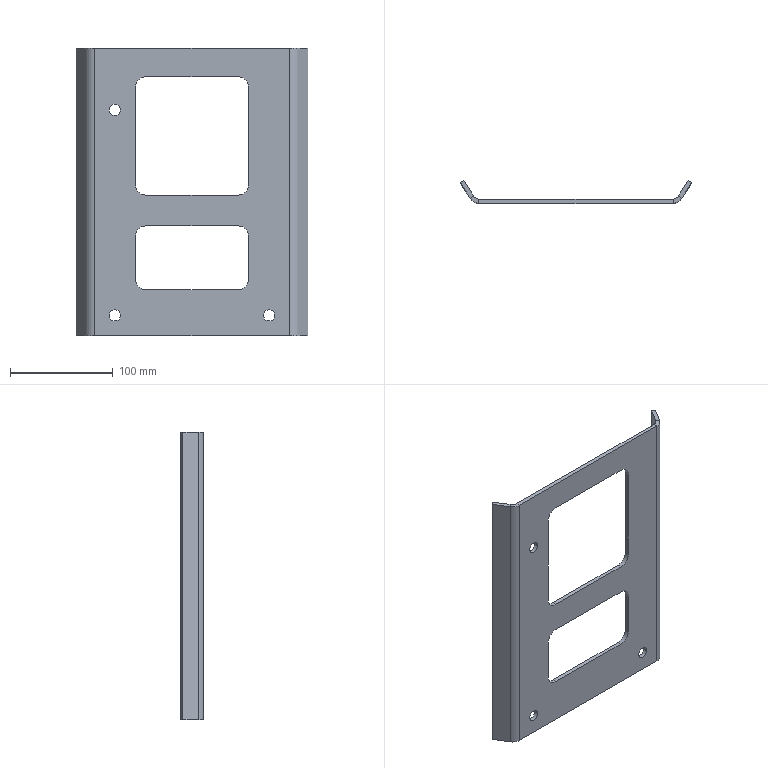Part | SolidWorks | features FlatPattern 1, ICE 1, SMBaseFlange 1, SheetMetal 1 | 1 solid | 44 faces | box 225 x 22.12 x 280 mm | volume 191805 mm3 | plane 26 | cylinder 18 | commonest cylinder face diameters 20 x10 11 x6 12 x2
STEP:
#1=CARTESIAN_POINT('',(182.,-16.,-120.));
#2=VERTEX_POINT('',#1);
#3=CARTESIAN_POINT('',(193.,-16.,-120.));
#4=VERTEX_POINT('',#3);
#5=CARTESIAN_POINT('',(187.5,-16.,-120.));
#6=DIRECTION('',(0.,-1.,0.));
#7=DIRECTION('',(-1.,0.,0.));
#8=AXIS2_PLACEMENT_3D('',#5,#6,#7);
#9=CIRCLE('',#8,5.5);
#10=EDGE_CURVE('',#2,#4,#9,.T.);
#11=ORIENTED_EDGE('',*,*,#10,.F.);
#12=CARTESIAN_POINT('',(182.,-20.,-120.));
#13=VERTEX_POINT('',#12);
#14=CARTESIAN_POINT('',(182.,2.121,-120.));
#15=DIRECTION('',(0.,-1.,0.));
#16=VECTOR('',#15,1000.);
#17=LINE('',#14,#16);
#18=EDGE_CURVE('',#2,#13,#17,.T.);
#19=ORIENTED_EDGE('',*,*,#18,.T.);
#20=CARTESIAN_POINT('',(193.,-20.,-120.));
#21=VERTEX_POINT('',#20);
#22=CARTESIAN_POINT('',(187.5,-20.,-120.));
#23=DIRECTION('',(0.,-1.,0.));
#24=DIRECTION('',(1.,0.,0.));
#25=AXIS2_PLACEMENT_3D('',#22,#23,#24);
#26=CIRCLE('',#25,5.5);
#27=EDGE_CURVE('',#13,#21,#26,.T.);
#28=ORIENTED_EDGE('',*,*,#27,.T.);
#29=CARTESIAN_POINT('',(193.,2.121,-120.));
#30=DIRECTION('',(0.,-1.,0.));
#31=VECTOR('',#30,1000.);
#32=LINE('',#29,#31);
#33=EDGE_CURVE('',#4,#21,#32,.T.);
#34=ORIENTED_EDGE('',*,*,#33,.F.);
#35=EDGE_LOOP('',(#11,#19,#28,#34));
#36=FACE_OUTER_BOUND('',#35,.T.);
#37=CARTESIAN_POINT('',(187.5,2.121,-120.));
#38=DIRECTION('',(0.,-1.,0.));
#39=DIRECTION('',(1.,0.,0.));
#40=AXIS2_PLACEMENT_3D('',#37,#38,#39);
#41=CYLINDRICAL_SURFACE('',#40,5.5);
#42=ADVANCED_FACE('',(#36),#41,.F.);
#43=CARTESIAN_POINT('',(32.,-16.,80.));
#44=VERTEX_POINT('',#43);
#45=CARTESIAN_POINT('',(43.,-16.,80.));
#46=VERTEX_POINT('',#45);
#47=CARTESIAN_POINT('',(37.5,-16.,80.));
#48=DIRECTION('',(0.,-1.,0.));
#49=DIRECTION('',(-1.,0.,0.));
#50=AXIS2_PLACEMENT_3D('',#47,#48,#49);
#51=CIRCLE('',#50,5.5);
#52=EDGE_CURVE('',#44,#46,#51,.T.);
#53=ORIENTED_EDGE('',*,*,#52,.F.);
#54=CARTESIAN_POINT('',(32.,-20.,80.));
#55=VERTEX_POINT('',#54);
#56=CARTESIAN_POINT('',(32.,2.121,80.));
#57=DIRECTION('',(0.,-1.,0.));
#58=VECTOR('',#57,1000.);
#59=LINE('',#56,#58);
#60=EDGE_CURVE('',#44,#55,#59,.T.);
#61=ORIENTED_EDGE('',*,*,#60,.T.);
#62=CARTESIAN_POINT('',(43.,-20.,80.));
#63=VERTEX_POINT('',#62);
#64=CARTESIAN_POINT('',(37.5,-20.,80.));
#65=DIRECTION('',(0.,-1.,0.));
#66=DIRECTION('',(1.,0.,0.));
#67=AXIS2_PLACEMENT_3D('',#64,#65,#66);
#68=CIRCLE('',#67,5.5);
#69=EDGE_CURVE('',#55,#63,#68,.T.);
#70=ORIENTED_EDGE('',*,*,#69,.T.);
#71=CARTESIAN_POINT('',(43.,2.121,80.));
#72=DIRECTION('',(0.,-1.,0.));
#73=VECTOR('',#72,1000.);
#74=LINE('',#71,#73);
#75=EDGE_CURVE('',#46,#63,#74,.T.);
#76=ORIENTED_EDGE('',*,*,#75,.F.);
#77=EDGE_LOOP('',(#53,#61,#70,#76));
#78=FACE_OUTER_BOUND('',#77,.T.);
#79=CARTESIAN_POINT('',(37.5,2.121,80.));
#80=DIRECTION('',(0.,-1.,0.));
#81=DIRECTION('',(1.,0.,0.));
#82=AXIS2_PLACEMENT_3D('',#79,#80,#81);
#83=CYLINDRICAL_SURFACE('',#82,5.5);
#84=ADVANCED_FACE('',(#78),#83,.F.);
#85=CARTESIAN_POINT('',(32.,-16.,-120.));
#86=VERTEX_POINT('',#85);
#87=CARTESIAN_POINT('',(43.,-16.,-120.));
#88=VERTEX_POINT('',#87);
#89=CARTESIAN_POINT('',(37.5,-16.,-120.));
#90=DIRECTION('',(0.,-1.,0.));
#91=DIRECTION('',(-1.,0.,0.));
#92=AXIS2_PLACEMENT_3D('',#89,#90,#91);
#93=CIRCLE('',#92,5.5);
#94=EDGE_CURVE('',#86,#88,#93,.T.);
#95=ORIENTED_EDGE('',*,*,#94,.F.);
#96=CARTESIAN_POINT('',(32.,-20.,-120.));
#97=VERTEX_POINT('',#96);
#98=CARTESIAN_POINT('',(32.,2.121,-120.));
#99=DIRECTION('',(0.,-1.,0.));
#100=VECTOR('',#99,1000.);
#101=LINE('',#98,#100);
#102=EDGE_CURVE('',#86,#97,#101,.T.);
#103=ORIENTED_EDGE('',*,*,#102,.T.);
#104=CARTESIAN_POINT('',(43.,-20.,-120.));
#105=VERTEX_POINT('',#104);
#106=CARTESIAN_POINT('',(37.5,-20.,-120.));
#107=DIRECTION('',(0.,-1.,0.));
#108=DIRECTION('',(1.,0.,0.));
#109=AXIS2_PLACEMENT_3D('',#106,#107,#108);
#110=CIRCLE('',#109,5.5);
#111=EDGE_CURVE('',#97,#105,#110,.T.);
#112=ORIENTED_EDGE('',*,*,#111,.T.);
#113=CARTESIAN_POINT('',(43.,2.121,-120.));
#114=DIRECTION('',(0.,-1.,0.));
#115=VECTOR('',#114,1000.);
#116=LINE('',#113,#115);
#117=EDGE_CURVE('',#88,#105,#116,.T.);
#118=ORIENTED_EDGE('',*,*,#117,.F.);
#119=EDGE_LOOP('',(#95,#103,#112,#118));
#120=FACE_OUTER_BOUND('',#119,.T.);
#121=CARTESIAN_POINT('',(37.5,2.121,-120.));
#122=DIRECTION('',(0.,-1.,0.));
#123=DIRECTION('',(1.,0.,0.));
#124=AXIS2_PLACEMENT_3D('',#121,#122,#123);
#125=CYLINDRICAL_SURFACE('',#124,5.5);
#126=ADVANCED_FACE('',(#120),#125,.F.);
#127=CARTESIAN_POINT('',(9.562,-15.3,140.));
#128=VERTEX_POINT('',#127);
#129=CARTESIAN_POINT('',(12.954,-13.18,140.));
#130=VERTEX_POINT('',#129);
#131=CARTESIAN_POINT('',(9.562,-15.3,140.));
#132=DIRECTION('',(0.848,0.53,0.));
#133=VECTOR('',#132,1000.);
#134=LINE('',#131,#133);
#135=EDGE_CURVE('',#128,#130,#134,.T.);
#136=ORIENTED_EDGE('',*,*,#135,.F.);
#137=CARTESIAN_POINT('',(18.042,-20.,140.));
#138=VERTEX_POINT('',#137);
#139=CARTESIAN_POINT('',(18.042,-10.,140.));
#140=DIRECTION('',(0.,0.,1.));
#141=DIRECTION('',(-1.,0.,0.));
#142=AXIS2_PLACEMENT_3D('',#139,#140,#141);
#143=CIRCLE('',#142,10.);
#144=EDGE_CURVE('',#128,#138,#143,.T.);
#145=ORIENTED_EDGE('',*,*,#144,.T.);
#146=CARTESIAN_POINT('',(18.042,-16.,140.));
#147=VERTEX_POINT('',#146);
#148=CARTESIAN_POINT('',(18.042,-16.,140.));
#149=DIRECTION('',(0.,-1.,0.));
#150=VECTOR('',#149,1000.);
#151=LINE('',#148,#150);
#152=EDGE_CURVE('',#147,#138,#151,.T.);
#153=ORIENTED_EDGE('',*,*,#152,.F.);
#154=CARTESIAN_POINT('',(18.042,-10.,140.));
#155=DIRECTION('',(0.,0.,1.));
#156=DIRECTION('',(1.,0.,0.));
#157=AXIS2_PLACEMENT_3D('',#154,#155,#156);
#158=CIRCLE('',#157,6.);
#159=EDGE_CURVE('',#130,#147,#158,.T.);
#160=ORIENTED_EDGE('',*,*,#159,.F.);
#161=EDGE_LOOP('',(#136,#145,#153,#160));
#162=FACE_OUTER_BOUND('',#161,.T.);
#163=CARTESIAN_POINT('',(9.562,-15.3,140.));
#164=DIRECTION('',(0.,0.,1.));
#165=DIRECTION('',(1.,0.,0.));
#166=AXIS2_PLACEMENT_3D('',#163,#164,#165);
#167=PLANE('',#166);
#168=ADVANCED_FACE('',(#162),#167,.T.);
#169=CARTESIAN_POINT('',(0.,0.,140.));
#170=VERTEX_POINT('',#169);
#171=CARTESIAN_POINT('',(0.,0.,140.));
#172=DIRECTION('',(0.53,-0.848,0.));
#173=VECTOR('',#172,1000.);
#174=LINE('',#171,#173);
#175=EDGE_CURVE('',#170,#128,#174,.T.);
#176=ORIENTED_EDGE('',*,*,#175,.T.);
#177=ORIENTED_EDGE('',*,*,#135,.T.);
#178=CARTESIAN_POINT('',(3.392,2.12,140.));
#179=VERTEX_POINT('',#178);
#180=CARTESIAN_POINT('',(3.392,2.12,140.));
#181=DIRECTION('',(0.53,-0.848,0.));
#182=VECTOR('',#181,1000.);
#183=LINE('',#180,#182);
#184=EDGE_CURVE('',#179,#130,#183,.T.);
#185=ORIENTED_EDGE('',*,*,#184,.F.);
#186=CARTESIAN_POINT('',(0.,0.,140.));
#187=DIRECTION('',(0.848,0.53,0.));
#188=VECTOR('',#187,1000.);
#189=LINE('',#186,#188);
#190=EDGE_CURVE('',#170,#179,#189,.T.);
#191=ORIENTED_EDGE('',*,*,#190,.F.);
#192=EDGE_LOOP('',(#176,#177,#185,#191));
#193=FACE_OUTER_BOUND('',#192,.T.);
#194=CARTESIAN_POINT('',(18.042,-16.,140.));
#195=DIRECTION('',(0.,0.,1.));
#196=DIRECTION('',(1.,0.,0.));
#197=AXIS2_PLACEMENT_3D('',#194,#195,#196);
#198=PLANE('',#197);
#199=ADVANCED_FACE('',(#193),#198,.T.);
#200=CARTESIAN_POINT('',(18.042,-20.,-140.));
#201=VERTEX_POINT('',#200);
#202=CARTESIAN_POINT('',(18.042,-16.,-140.));
#203=VERTEX_POINT('',#202);
#204=CARTESIAN_POINT('',(18.042,-20.,-140.));
#205=DIRECTION('',(0.,1.,0.));
#206=VECTOR('',#205,1000.);
#207=LINE('',#204,#206);
#208=EDGE_CURVE('',#201,#203,#207,.T.);
#209=ORIENTED_EDGE('',*,*,#208,.F.);
#210=CARTESIAN_POINT('',(9.562,-15.3,-140.));
#211=VERTEX_POINT('',#210);
#212=CARTESIAN_POINT('',(18.042,-10.,-140.));
#213=DIRECTION('',(0.,0.,1.));
#214=DIRECTION('',(-1.,0.,0.));
#215=AXIS2_PLACEMENT_3D('',#212,#213,#214);
#216=CIRCLE('',#215,10.);
#217=EDGE_CURVE('',#211,#201,#216,.T.);
#218=ORIENTED_EDGE('',*,*,#217,.F.);
#219=CARTESIAN_POINT('',(12.954,-13.18,-140.));
#220=VERTEX_POINT('',#219);
#221=CARTESIAN_POINT('',(12.954,-13.18,-140.));
#222=DIRECTION('',(-0.848,-0.53,0.));
#223=VECTOR('',#222,1000.);
#224=LINE('',#221,#223);
#225=EDGE_CURVE('',#220,#211,#224,.T.);
#226=ORIENTED_EDGE('',*,*,#225,.F.);
#227=CARTESIAN_POINT('',(18.042,-10.,-140.));
#228=DIRECTION('',(0.,0.,1.));
#229=DIRECTION('',(1.,0.,0.));
#230=AXIS2_PLACEMENT_3D('',#227,#228,#229);
#231=CIRCLE('',#230,6.);
#232=EDGE_CURVE('',#220,#203,#231,.T.);
#233=ORIENTED_EDGE('',*,*,#232,.T.);
#234=EDGE_LOOP('',(#209,#218,#226,#233));
#235=FACE_OUTER_BOUND('',#234,.T.);
#236=CARTESIAN_POINT('',(18.042,-20.,-140.));
#237=DIRECTION('',(0.,0.,-1.));
#238=DIRECTION('',(-1.,0.,0.));
#239=AXIS2_PLACEMENT_3D('',#236,#237,#238);
#240=PLANE('',#239);
#241=ADVANCED_FACE('',(#235),#240,.T.);
#242=CARTESIAN_POINT('',(206.958,-20.,-140.));
#243=VERTEX_POINT('',#242);
#244=CARTESIAN_POINT('',(12.5,-20.,-140.));
#245=DIRECTION('',(1.,0.,0.));
#246=VECTOR('',#245,1000.);
#247=LINE('',#244,#246);
#248=EDGE_CURVE('',#201,#243,#247,.T.);
#249=ORIENTED_EDGE('',*,*,#248,.F.);
#250=ORIENTED_EDGE('',*,*,#208,.T.);
#251=CARTESIAN_POINT('',(206.958,-16.,-140.));
#252=VERTEX_POINT('',#251);
#253=CARTESIAN_POINT('',(12.5,-16.,-140.));
#254=DIRECTION('',(1.,0.,0.));
#255=VECTOR('',#254,1000.);
#256=LINE('',#253,#255);
#257=EDGE_CURVE('',#203,#252,#256,.T.);
#258=ORIENTED_EDGE('',*,*,#257,.T.);
#259=CARTESIAN_POINT('',(206.958,-16.,-140.));
#260=DIRECTION('',(0.,-1.,0.));
#261=VECTOR('',#260,1000.);
#262=LINE('',#259,#261);
#263=EDGE_CURVE('',#252,#243,#262,.T.);
#264=ORIENTED_EDGE('',*,*,#263,.T.);
#265=EDGE_LOOP('',(#249,#250,#258,#264));
#266=FACE_OUTER_BOUND('',#265,.T.);
#267=CARTESIAN_POINT('',(12.954,-13.18,-140.));
#268=DIRECTION('',(0.,0.,-1.));
#269=DIRECTION('',(-1.,0.,0.));
#270=AXIS2_PLACEMENT_3D('',#267,#268,#269);
#271=PLANE('',#270);
#272=ADVANCED_FACE('',(#266),#271,.T.);
#273=CARTESIAN_POINT('',(206.958,-20.,140.));
#274=VERTEX_POINT('',#273);
#275=CARTESIAN_POINT('',(206.958,-16.,140.));
#276=VERTEX_POINT('',#275);
#277=CARTESIAN_POINT('',(206.958,-20.,140.));
#278=DIRECTION('',(0.,1.,0.));
#279=VECTOR('',#278,1000.);
#280=LINE('',#277,#279);
#281=EDGE_CURVE('',#274,#276,#280,.T.);
#282=ORIENTED_EDGE('',*,*,#281,.F.);
#283=CARTESIAN_POINT('',(215.438,-15.3,140.));
#284=VERTEX_POINT('',#283);
#285=CARTESIAN_POINT('',(206.958,-10.,140.));
#286=DIRECTION('',(0.,0.,1.));
#287=DIRECTION('',(-1.,0.,0.));
#288=AXIS2_PLACEMENT_3D('',#285,#286,#287);
#289=CIRCLE('',#288,10.);
#290=EDGE_CURVE('',#274,#284,#289,.T.);
#291=ORIENTED_EDGE('',*,*,#290,.T.);
#292=CARTESIAN_POINT('',(212.046,-13.18,140.));
#293=VERTEX_POINT('',#292);
#294=CARTESIAN_POINT('',(212.046,-13.18,140.));
#295=DIRECTION('',(0.848,-0.53,0.));
#296=VECTOR('',#295,1000.);
#297=LINE('',#294,#296);
#298=EDGE_CURVE('',#293,#284,#297,.T.);
#299=ORIENTED_EDGE('',*,*,#298,.F.);
#300=CARTESIAN_POINT('',(206.958,-10.,140.));
#301=DIRECTION('',(0.,0.,1.));
#302=DIRECTION('',(1.,0.,0.));
#303=AXIS2_PLACEMENT_3D('',#300,#301,#302);
#304=CIRCLE('',#303,6.);
#305=EDGE_CURVE('',#276,#293,#304,.T.);
#306=ORIENTED_EDGE('',*,*,#305,.F.);
#307=EDGE_LOOP('',(#282,#291,#299,#306));
#308=FACE_OUTER_BOUND('',#307,.T.);
#309=CARTESIAN_POINT('',(206.958,-20.,140.));
#310=DIRECTION('',(0.,0.,1.));
#311=DIRECTION('',(1.,0.,0.));
#312=AXIS2_PLACEMENT_3D('',#309,#310,#311);
#313=PLANE('',#312);
#314=ADVANCED_FACE('',(#308),#313,.T.);
#315=CARTESIAN_POINT('',(12.5,-20.,140.));
#316=DIRECTION('',(1.,0.,0.));
#317=VECTOR('',#316,1000.);
#318=LINE('',#315,#317);
#319=EDGE_CURVE('',#138,#274,#318,.T.);
#320=ORIENTED_EDGE('',*,*,#319,.T.);
#321=ORIENTED_EDGE('',*,*,#281,.T.);
#322=CARTESIAN_POINT('',(12.5,-16.,140.));
#323=DIRECTION('',(1.,0.,0.));
#324=VECTOR('',#323,1000.);
#325=LINE('',#322,#324);
#326=EDGE_CURVE('',#147,#276,#325,.T.);
#327=ORIENTED_EDGE('',*,*,#326,.F.);
#328=ORIENTED_EDGE('',*,*,#152,.T.);
#329=EDGE_LOOP('',(#320,#321,#327,#328));
#330=FACE_OUTER_BOUND('',#329,.T.);
#331=CARTESIAN_POINT('',(212.046,-13.18,140.));
#332=DIRECTION('',(0.,0.,1.));
#333=DIRECTION('',(1.,0.,0.));
#334=AXIS2_PLACEMENT_3D('',#331,#332,#333);
#335=PLANE('',#334);
#336=ADVANCED_FACE('',(#330),#335,.T.);
#337=CARTESIAN_POINT('',(215.438,-15.3,-140.));
#338=VERTEX_POINT('',#337);
#339=CARTESIAN_POINT('',(212.046,-13.18,-140.));
#340=VERTEX_POINT('',#339);
#341=CARTESIAN_POINT('',(215.438,-15.3,-140.));
#342=DIRECTION('',(-0.848,0.53,0.));
#343=VECTOR('',#342,1000.);
#344=LINE('',#341,#343);
#345=EDGE_CURVE('',#338,#340,#344,.T.);
#346=ORIENTED_EDGE('',*,*,#345,.F.);
#347=CARTESIAN_POINT('',(206.958,-10.,-140.));
#348=DIRECTION('',(0.,0.,1.));
#349=DIRECTION('',(-1.,0.,0.));
#350=AXIS2_PLACEMENT_3D('',#347,#348,#349);
#351=CIRCLE('',#350,10.);
#352=EDGE_CURVE('',#243,#338,#351,.T.);
#353=ORIENTED_EDGE('',*,*,#352,.F.);
#354=ORIENTED_EDGE('',*,*,#263,.F.);
#355=CARTESIAN_POINT('',(206.958,-10.,-140.));
#356=DIRECTION('',(0.,0.,1.));
#357=DIRECTION('',(1.,0.,0.));
#358=AXIS2_PLACEMENT_3D('',#355,#356,#357);
#359=CIRCLE('',#358,6.);
#360=EDGE_CURVE('',#252,#340,#359,.T.);
#361=ORIENTED_EDGE('',*,*,#360,.T.);
#362=EDGE_LOOP('',(#346,#353,#354,#361));
#363=FACE_OUTER_BOUND('',#362,.T.);
#364=CARTESIAN_POINT('',(215.438,-15.3,-140.));
#365=DIRECTION('',(0.,0.,-1.));
#366=DIRECTION('',(-1.,0.,0.));
#367=AXIS2_PLACEMENT_3D('',#364,#365,#366);
#368=PLANE('',#367);
#369=ADVANCED_FACE('',(#363),#368,.T.);
#370=CARTESIAN_POINT('',(225.,0.,-140.));
#371=VERTEX_POINT('',#370);
#372=CARTESIAN_POINT('',(212.5,-20.,-140.));
#373=DIRECTION('',(0.53,0.848,0.));
#374=VECTOR('',#373,1000.);
#375=LINE('',#372,#374);
#376=EDGE_CURVE('',#338,#371,#375,.T.);
#377=ORIENTED_EDGE('',*,*,#376,.F.);
#378=ORIENTED_EDGE('',*,*,#345,.T.);
#379=CARTESIAN_POINT('',(221.608,2.12,-140.));
#380=VERTEX_POINT('',#379);
#381=CARTESIAN_POINT('',(209.108,-17.88,-140.));
#382=DIRECTION('',(0.53,0.848,0.));
#383=VECTOR('',#382,1000.);
#384=LINE('',#381,#383);
#385=EDGE_CURVE('',#340,#380,#384,.T.);
#386=ORIENTED_EDGE('',*,*,#385,.T.);
#387=CARTESIAN_POINT('',(221.608,2.12,-140.));
#388=DIRECTION('',(0.848,-0.53,0.));
#389=VECTOR('',#388,1000.);
#390=LINE('',#387,#389);
#391=EDGE_CURVE('',#380,#371,#390,.T.);
#392=ORIENTED_EDGE('',*,*,#391,.T.);
#393=EDGE_LOOP('',(#377,#378,#386,#392));
#394=FACE_OUTER_BOUND('',#393,.T.);
#395=CARTESIAN_POINT('',(206.958,-16.,-140.));
#396=DIRECTION('',(0.,0.,-1.));
#397=DIRECTION('',(-1.,0.,0.));
#398=AXIS2_PLACEMENT_3D('',#395,#396,#397);
#399=PLANE('',#398);
#400=ADVANCED_FACE('',(#394),#399,.T.);
#401=ORIENTED_EDGE('',*,*,#376,.T.);
#402=CARTESIAN_POINT('',(225.,0.,140.));
#403=VERTEX_POINT('',#402);
#404=CARTESIAN_POINT('',(225.,0.,140.));
#405=DIRECTION('',(0.,0.,-1.));
#406=VECTOR('',#405,1000.);
#407=LINE('',#404,#406);
#408=EDGE_CURVE('',#403,#371,#407,.T.);
#409=ORIENTED_EDGE('',*,*,#408,.F.);
#410=CARTESIAN_POINT('',(212.5,-20.,140.));
#411=DIRECTION('',(0.53,0.848,0.));
#412=VECTOR('',#411,1000.);
#413=LINE('',#410,#412);
#414=EDGE_CURVE('',#284,#403,#413,.T.);
#415=ORIENTED_EDGE('',*,*,#414,.F.);
#416=CARTESIAN_POINT('',(215.438,-15.3,140.));
#417=DIRECTION('',(0.,0.,-1.));
#418=VECTOR('',#417,1000.);
#419=LINE('',#416,#418);
#420=EDGE_CURVE('',#284,#338,#419,.T.);
#421=ORIENTED_EDGE('',*,*,#420,.T.);
#422=EDGE_LOOP('',(#401,#409,#415,#421));
#423=FACE_OUTER_BOUND('',#422,.T.);
#424=CARTESIAN_POINT('',(212.5,-20.,140.));
#425=DIRECTION('',(-0.848,0.53,0.));
#426=DIRECTION('',(-0.53,-0.848,0.));
#427=AXIS2_PLACEMENT_3D('',#424,#425,#426);
#428=PLANE('',#427);
#429=ADVANCED_FACE('',(#423),#428,.F.);
#430=ORIENTED_EDGE('',*,*,#391,.F.);
#431=CARTESIAN_POINT('',(221.608,2.12,140.));
#432=VERTEX_POINT('',#431);
#433=CARTESIAN_POINT('',(221.608,2.12,140.));
#434=DIRECTION('',(0.,0.,-1.));
#435=VECTOR('',#434,1000.);
#436=LINE('',#433,#435);
#437=EDGE_CURVE('',#432,#380,#436,.T.);
#438=ORIENTED_EDGE('',*,*,#437,.F.);
#439=CARTESIAN_POINT('',(221.608,2.12,140.));
#440=DIRECTION('',(0.848,-0.53,0.));
#441=VECTOR('',#440,1000.);
#442=LINE('',#439,#441);
#443=EDGE_CURVE('',#432,#403,#442,.T.);
#444=ORIENTED_EDGE('',*,*,#443,.T.);
#445=ORIENTED_EDGE('',*,*,#408,.T.);
#446=EDGE_LOOP('',(#430,#438,#444,#445));
#447=FACE_OUTER_BOUND('',#446,.T.);
#448=CARTESIAN_POINT('',(221.608,2.12,140.));
#449=DIRECTION('',(0.53,0.848,0.));
#450=DIRECTION('',(-0.848,0.53,0.));
#451=AXIS2_PLACEMENT_3D('',#448,#449,#450);
#452=PLANE('',#451);
#453=ADVANCED_FACE('',(#447),#452,.T.);
#454=ORIENTED_EDGE('',*,*,#385,.F.);
#455=CARTESIAN_POINT('',(212.046,-13.18,140.));
#456=DIRECTION('',(0.,0.,-1.));
#457=VECTOR('',#456,1000.);
#458=LINE('',#455,#457);
#459=EDGE_CURVE('',#293,#340,#458,.T.);
#460=ORIENTED_EDGE('',*,*,#459,.F.);
#461=CARTESIAN_POINT('',(209.108,-17.88,140.));
#462=DIRECTION('',(0.53,0.848,0.));
#463=VECTOR('',#462,1000.);
#464=LINE('',#461,#463);
#465=EDGE_CURVE('',#293,#432,#464,.T.);
#466=ORIENTED_EDGE('',*,*,#465,.T.);
#467=ORIENTED_EDGE('',*,*,#437,.T.);
#468=EDGE_LOOP('',(#454,#460,#466,#467));
#469=FACE_OUTER_BOUND('',#468,.T.);
#470=CARTESIAN_POINT('',(209.108,-17.88,140.));
#471=DIRECTION('',(-0.848,0.53,0.));
#472=DIRECTION('',(-0.53,-0.848,0.));
#473=AXIS2_PLACEMENT_3D('',#470,#471,#472);
#474=PLANE('',#473);
#475=ADVANCED_FACE('',(#469),#474,.T.);
#476=ORIENTED_EDGE('',*,*,#360,.F.);
#477=CARTESIAN_POINT('',(206.958,-16.,140.));
#478=DIRECTION('',(0.,0.,-1.));
#479=VECTOR('',#478,1000.);
#480=LINE('',#477,#479);
#481=EDGE_CURVE('',#276,#252,#480,.T.);
#482=ORIENTED_EDGE('',*,*,#481,.F.);
#483=ORIENTED_EDGE('',*,*,#305,.T.);
#484=ORIENTED_EDGE('',*,*,#459,.T.);
#485=EDGE_LOOP('',(#476,#482,#483,#484));
#486=FACE_OUTER_BOUND('',#485,.T.);
#487=CARTESIAN_POINT('',(206.958,-10.,140.));
#488=DIRECTION('',(0.,0.,-1.));
#489=DIRECTION('',(-1.,0.,0.));
#490=AXIS2_PLACEMENT_3D('',#487,#488,#489);
#491=CYLINDRICAL_SURFACE('',#490,6.);
#492=ADVANCED_FACE('',(#486),#491,.F.);
#493=CARTESIAN_POINT('',(187.5,-16.,-120.));
#494=DIRECTION('',(0.,-1.,0.));
#495=DIRECTION('',(-1.,0.,0.));
#496=AXIS2_PLACEMENT_3D('',#493,#494,#495);
#497=CIRCLE('',#496,5.5);
#498=EDGE_CURVE('',#4,#2,#497,.T.);
#499=ORIENTED_EDGE('',*,*,#498,.T.);
#500=ORIENTED_EDGE('',*,*,#10,.T.);
#501=EDGE_LOOP('',(#499,#500));
#502=FACE_BOUND('',#501,.T.);
#503=CARTESIAN_POINT('',(37.5,-16.,80.));
#504=DIRECTION('',(0.,-1.,0.));
#505=DIRECTION('',(-1.,0.,0.));
#506=AXIS2_PLACEMENT_3D('',#503,#504,#505);
#507=CIRCLE('',#506,5.5);
#508=EDGE_CURVE('',#46,#44,#507,.T.);
#509=ORIENTED_EDGE('',*,*,#508,.T.);
#510=ORIENTED_EDGE('',*,*,#52,.T.);
#511=EDGE_LOOP('',(#509,#510));
#512=FACE_BOUND('',#511,.T.);
#513=CARTESIAN_POINT('',(57.5,-16.,-85.));
#514=VERTEX_POINT('',#513);
#515=CARTESIAN_POINT('',(67.5,-16.,-95.));
#516=VERTEX_POINT('',#515);
#517=CARTESIAN_POINT('',(67.5,-16.,-85.));
#518=DIRECTION('',(0.,-1.,0.));
#519=DIRECTION('',(-1.,0.,0.));
#520=AXIS2_PLACEMENT_3D('',#517,#518,#519);
#521=CIRCLE('',#520,10.);
#522=EDGE_CURVE('',#514,#516,#521,.T.);
#523=ORIENTED_EDGE('',*,*,#522,.T.);
#524=CARTESIAN_POINT('',(157.5,-16.,-95.));
#525=VERTEX_POINT('',#524);
#526=CARTESIAN_POINT('',(67.5,-16.,-95.));
#527=DIRECTION('',(1.,0.,0.));
#528=VECTOR('',#527,1000.);
#529=LINE('',#526,#528);
#530=EDGE_CURVE('',#516,#525,#529,.T.);
#531=ORIENTED_EDGE('',*,*,#530,.T.);
#532=CARTESIAN_POINT('',(167.5,-16.,-85.));
#533=VERTEX_POINT('',#532);
#534=CARTESIAN_POINT('',(157.5,-16.,-85.));
#535=DIRECTION('',(0.,-1.,0.));
#536=DIRECTION('',(-1.,0.,0.));
#537=AXIS2_PLACEMENT_3D('',#534,#535,#536);
#538=CIRCLE('',#537,10.);
#539=EDGE_CURVE('',#525,#533,#538,.T.);
#540=ORIENTED_EDGE('',*,*,#539,.T.);
#541=CARTESIAN_POINT('',(167.5,-16.,-43.));
#542=VERTEX_POINT('',#541);
#543=CARTESIAN_POINT('',(167.5,-16.,-43.));
#544=DIRECTION('',(0.,0.,1.));
#545=VECTOR('',#544,1000.);
#546=LINE('',#543,#545);
#547=EDGE_CURVE('',#533,#542,#546,.T.);
#548=ORIENTED_EDGE('',*,*,#547,.T.);
#549=CARTESIAN_POINT('',(157.5,-16.,-33.));
#550=VERTEX_POINT('',#549);
#551=CARTESIAN_POINT('',(157.5,-16.,-43.));
#552=DIRECTION('',(0.,-1.,0.));
#553=DIRECTION('',(-1.,0.,0.));
#554=AXIS2_PLACEMENT_3D('',#551,#552,#553);
#555=CIRCLE('',#554,10.);
#556=EDGE_CURVE('',#542,#550,#555,.T.);
#557=ORIENTED_EDGE('',*,*,#556,.T.);
#558=CARTESIAN_POINT('',(67.5,-16.,-33.));
#559=VERTEX_POINT('',#558);
#560=CARTESIAN_POINT('',(67.5,-16.,-33.));
#561=DIRECTION('',(-1.,0.,0.));
#562=VECTOR('',#561,1000.);
#563=LINE('',#560,#562);
#564=EDGE_CURVE('',#550,#559,#563,.T.);
#565=ORIENTED_EDGE('',*,*,#564,.T.);
#566=CARTESIAN_POINT('',(57.5,-16.,-43.));
#567=VERTEX_POINT('',#566);
#568=CARTESIAN_POINT('',(67.5,-16.,-43.));
#569=DIRECTION('',(0.,-1.,0.));
#570=DIRECTION('',(-1.,0.,0.));
#571=AXIS2_PLACEMENT_3D('',#568,#569,#570);
#572=CIRCLE('',#571,10.);
#573=EDGE_CURVE('',#559,#567,#572,.T.);
#574=ORIENTED_EDGE('',*,*,#573,.T.);
#575=CARTESIAN_POINT('',(57.5,-16.,-43.));
#576=DIRECTION('',(0.,0.,-1.));
#577=VECTOR('',#576,1000.);
#578=LINE('',#575,#577);
#579=EDGE_CURVE('',#567,#514,#578,.T.);
#580=ORIENTED_EDGE('',*,*,#579,.T.);
#581=EDGE_LOOP('',(#523,#531,#540,#548,#557,#565,#574,#580));
#582=FACE_BOUND('',#581,.T.);
#583=CARTESIAN_POINT('',(57.5,-16.,7.));
#584=VERTEX_POINT('',#583);
#585=CARTESIAN_POINT('',(67.5,-16.,-3.));
#586=VERTEX_POINT('',#585);
#587=CARTESIAN_POINT('',(67.5,-16.,7.));
#588=DIRECTION('',(0.,-1.,0.));
#589=DIRECTION('',(-1.,0.,0.));
#590=AXIS2_PLACEMENT_3D('',#587,#588,#589);
#591=CIRCLE('',#590,10.);
#592=EDGE_CURVE('',#584,#586,#591,.T.);
#593=ORIENTED_EDGE('',*,*,#592,.T.);
#594=CARTESIAN_POINT('',(157.5,-16.,-3.));
#595=VERTEX_POINT('',#594);
#596=CARTESIAN_POINT('',(67.5,-16.,-3.));
#597=DIRECTION('',(1.,0.,0.));
#598=VECTOR('',#597,1000.);
#599=LINE('',#596,#598);
#600=EDGE_CURVE('',#586,#595,#599,.T.);
#601=ORIENTED_EDGE('',*,*,#600,.T.);
#602=CARTESIAN_POINT('',(167.5,-16.,7.));
#603=VERTEX_POINT('',#602);
#604=CARTESIAN_POINT('',(157.5,-16.,7.));
#605=DIRECTION('',(0.,-1.,0.));
#606=DIRECTION('',(-1.,0.,0.));
#607=AXIS2_PLACEMENT_3D('',#604,#605,#606);
#608=CIRCLE('',#607,10.);
#609=EDGE_CURVE('',#595,#603,#608,.T.);
#610=ORIENTED_EDGE('',*,*,#609,.T.);
#611=CARTESIAN_POINT('',(167.5,-16.,102.));
#612=VERTEX_POINT('',#611);
#613=CARTESIAN_POINT('',(167.5,-16.,102.));
#614=DIRECTION('',(0.,0.,1.));
#615=VECTOR('',#614,1000.);
#616=LINE('',#613,#615);
#617=EDGE_CURVE('',#603,#612,#616,.T.);
#618=ORIENTED_EDGE('',*,*,#617,.T.);
#619=CARTESIAN_POINT('',(157.5,-16.,112.));
#620=VERTEX_POINT('',#619);
#621=CARTESIAN_POINT('',(157.5,-16.,102.));
#622=DIRECTION('',(0.,-1.,0.));
#623=DIRECTION('',(-1.,0.,0.));
#624=AXIS2_PLACEMENT_3D('',#621,#622,#623);
#625=CIRCLE('',#624,10.);
#626=EDGE_CURVE('',#612,#620,#625,.T.);
#627=ORIENTED_EDGE('',*,*,#626,.T.);
#628=CARTESIAN_POINT('',(67.5,-16.,112.));
#629=VERTEX_POINT('',#628);
#630=CARTESIAN_POINT('',(67.5,-16.,112.));
#631=DIRECTION('',(-1.,0.,0.));
#632=VECTOR('',#631,1000.);
#633=LINE('',#630,#632);
#634=EDGE_CURVE('',#620,#629,#633,.T.);
#635=ORIENTED_EDGE('',*,*,#634,.T.);
#636=CARTESIAN_POINT('',(57.5,-16.,102.));
#637=VERTEX_POINT('',#636);
#638=CARTESIAN_POINT('',(67.5,-16.,102.));
#639=DIRECTION('',(0.,-1.,0.));
#640=DIRECTION('',(-1.,0.,0.));
#641=AXIS2_PLACEMENT_3D('',#638,#639,#640);
#642=CIRCLE('',#641,10.);
#643=EDGE_CURVE('',#629,#637,#642,.T.);
#644=ORIENTED_EDGE('',*,*,#643,.T.);
#645=CARTESIAN_POINT('',(57.5,-16.,102.));
#646=DIRECTION('',(0.,0.,-1.));
#647=VECTOR('',#646,1000.);
#648=LINE('',#645,#647);
#649=EDGE_CURVE('',#637,#584,#648,.T.);
#650=ORIENTED_EDGE('',*,*,#649,.T.);
#651=EDGE_LOOP('',(#593,#601,#610,#618,#627,#635,#644,#650));
#652=FACE_BOUND('',#651,.T.);
#653=CARTESIAN_POINT('',(37.5,-16.,-120.));
#654=DIRECTION('',(0.,-1.,0.));
#655=DIRECTION('',(-1.,0.,0.));
#656=AXIS2_PLACEMENT_3D('',#653,#654,#655);
#657=CIRCLE('',#656,5.5);
#658=EDGE_CURVE('',#88,#86,#657,.T.);
#659=ORIENTED_EDGE('',*,*,#658,.T.);
#660=ORIENTED_EDGE('',*,*,#94,.T.);
#661=EDGE_LOOP('',(#659,#660));
#662=FACE_BOUND('',#661,.T.);
#663=ORIENTED_EDGE('',*,*,#257,.F.);
#664=CARTESIAN_POINT('',(18.042,-16.,140.));
#665=DIRECTION('',(0.,0.,-1.));
#666=VECTOR('',#665,1000.);
#667=LINE('',#664,#666);
#668=EDGE_CURVE('',#147,#203,#667,.T.);
#669=ORIENTED_EDGE('',*,*,#668,.F.);
#670=ORIENTED_EDGE('',*,*,#326,.T.);
#671=ORIENTED_EDGE('',*,*,#481,.T.);
#672=EDGE_LOOP('',(#663,#669,#670,#671));
#673=FACE_OUTER_BOUND('',#672,.T.);
#674=CARTESIAN_POINT('',(12.5,-16.,140.));
#675=DIRECTION('',(0.,1.,0.));
#676=DIRECTION('',(-1.,0.,0.));
#677=AXIS2_PLACEMENT_3D('',#674,#675,#676);
#678=PLANE('',#677);
#679=ADVANCED_FACE('',(#502,#512,#582,#652,#662,#673),#678,.T.);
#680=ORIENTED_EDGE('',*,*,#232,.F.);
#681=CARTESIAN_POINT('',(12.954,-13.18,140.));
#682=DIRECTION('',(0.,0.,-1.));
#683=VECTOR('',#682,1000.);
#684=LINE('',#681,#683);
#685=EDGE_CURVE('',#130,#220,#684,.T.);
#686=ORIENTED_EDGE('',*,*,#685,.F.);
#687=ORIENTED_EDGE('',*,*,#159,.T.);
#688=ORIENTED_EDGE('',*,*,#668,.T.);
#689=EDGE_LOOP('',(#680,#686,#687,#688));
#690=FACE_OUTER_BOUND('',#689,.T.);
#691=CARTESIAN_POINT('',(18.042,-10.,140.));
#692=DIRECTION('',(0.,0.,-1.));
#693=DIRECTION('',(-1.,0.,0.));
#694=AXIS2_PLACEMENT_3D('',#691,#692,#693);
#695=CYLINDRICAL_SURFACE('',#694,6.);
#696=ADVANCED_FACE('',(#690),#695,.F.);
#697=CARTESIAN_POINT('',(3.392,2.12,-140.));
#698=VERTEX_POINT('',#697);
#699=CARTESIAN_POINT('',(3.392,2.12,-140.));
#700=DIRECTION('',(0.53,-0.848,0.));
#701=VECTOR('',#700,1000.);
#702=LINE('',#699,#701);
#703=EDGE_CURVE('',#698,#220,#702,.T.);
#704=ORIENTED_EDGE('',*,*,#703,.F.);
#705=CARTESIAN_POINT('',(3.392,2.12,140.));
#706=DIRECTION('',(0.,0.,-1.));
#707=VECTOR('',#706,1000.);
#708=LINE('',#705,#707);
#709=EDGE_CURVE('',#179,#698,#708,.T.);
#710=ORIENTED_EDGE('',*,*,#709,.F.);
#711=ORIENTED_EDGE('',*,*,#184,.T.);
#712=ORIENTED_EDGE('',*,*,#685,.T.);
#713=EDGE_LOOP('',(#704,#710,#711,#712));
#714=FACE_OUTER_BOUND('',#713,.T.);
#715=CARTESIAN_POINT('',(3.392,2.12,140.));
#716=DIRECTION('',(0.848,0.53,0.));
#717=DIRECTION('',(-0.53,0.848,0.));
#718=AXIS2_PLACEMENT_3D('',#715,#716,#717);
#719=PLANE('',#718);
#720=ADVANCED_FACE('',(#714),#719,.T.);
#721=CARTESIAN_POINT('',(0.,0.,-140.));
#722=VERTEX_POINT('',#721);
#723=CARTESIAN_POINT('',(0.,0.,-140.));
#724=DIRECTION('',(0.848,0.53,0.));
#725=VECTOR('',#724,1000.);
#726=LINE('',#723,#725);
#727=EDGE_CURVE('',#722,#698,#726,.T.);
#728=ORIENTED_EDGE('',*,*,#727,.F.);
#729=CARTESIAN_POINT('',(0.,0.,140.));
#730=DIRECTION('',(0.,0.,-1.));
#731=VECTOR('',#730,1000.);
#732=LINE('',#729,#731);
#733=EDGE_CURVE('',#170,#722,#732,.T.);
#734=ORIENTED_EDGE('',*,*,#733,.F.);
#735=ORIENTED_EDGE('',*,*,#190,.T.);
#736=ORIENTED_EDGE('',*,*,#709,.T.);
#737=EDGE_LOOP('',(#728,#734,#735,#736));
#738=FACE_OUTER_BOUND('',#737,.T.);
#739=CARTESIAN_POINT('',(0.,0.,140.));
#740=DIRECTION('',(-0.53,0.848,0.));
#741=DIRECTION('',(-0.848,-0.53,0.));
#742=AXIS2_PLACEMENT_3D('',#739,#740,#741);
#743=PLANE('',#742);
#744=ADVANCED_FACE('',(#738),#743,.T.);
#745=CARTESIAN_POINT('',(0.,0.,-140.));
#746=DIRECTION('',(0.53,-0.848,0.));
#747=VECTOR('',#746,1000.);
#748=LINE('',#745,#747);
#749=EDGE_CURVE('',#722,#211,#748,.T.);
#750=ORIENTED_EDGE('',*,*,#749,.T.);
#751=CARTESIAN_POINT('',(9.562,-15.3,140.));
#752=DIRECTION('',(0.,0.,-1.));
#753=VECTOR('',#752,1000.);
#754=LINE('',#751,#753);
#755=EDGE_CURVE('',#128,#211,#754,.T.);
#756=ORIENTED_EDGE('',*,*,#755,.F.);
#757=ORIENTED_EDGE('',*,*,#175,.F.);
#758=ORIENTED_EDGE('',*,*,#733,.T.);
#759=EDGE_LOOP('',(#750,#756,#757,#758));
#760=FACE_OUTER_BOUND('',#759,.T.);
#761=CARTESIAN_POINT('',(0.,0.,140.));
#762=DIRECTION('',(0.848,0.53,0.));
#763=DIRECTION('',(-0.53,0.848,0.));
#764=AXIS2_PLACEMENT_3D('',#761,#762,#763);
#765=PLANE('',#764);
#766=ADVANCED_FACE('',(#760),#765,.F.);
#767=ORIENTED_EDGE('',*,*,#217,.T.);
#768=CARTESIAN_POINT('',(18.042,-20.,140.));
#769=DIRECTION('',(0.,0.,-1.));
#770=VECTOR('',#769,1000.);
#771=LINE('',#768,#770);
#772=EDGE_CURVE('',#138,#201,#771,.T.);
#773=ORIENTED_EDGE('',*,*,#772,.F.);
#774=ORIENTED_EDGE('',*,*,#144,.F.);
#775=ORIENTED_EDGE('',*,*,#755,.T.);
#776=EDGE_LOOP('',(#767,#773,#774,#775));
#777=FACE_OUTER_BOUND('',#776,.T.);
#778=CARTESIAN_POINT('',(18.042,-10.,140.));
#779=DIRECTION('',(0.,0.,-1.));
#780=DIRECTION('',(-1.,0.,0.));
#781=AXIS2_PLACEMENT_3D('',#778,#779,#780);
#782=CYLINDRICAL_SURFACE('',#781,10.);
#783=ADVANCED_FACE('',(#777),#782,.T.);
#784=CARTESIAN_POINT('',(187.5,-20.,-120.));
#785=DIRECTION('',(0.,-1.,0.));
#786=DIRECTION('',(1.,0.,0.));
#787=AXIS2_PLACEMENT_3D('',#784,#785,#786);
#788=CIRCLE('',#787,5.5);
#789=EDGE_CURVE('',#21,#13,#788,.T.);
#790=ORIENTED_EDGE('',*,*,#789,.F.);
#791=ORIENTED_EDGE('',*,*,#27,.F.);
#792=EDGE_LOOP('',(#790,#791));
#793=FACE_BOUND('',#792,.T.);
#794=CARTESIAN_POINT('',(37.5,-20.,80.));
#795=DIRECTION('',(0.,-1.,0.));
#796=DIRECTION('',(1.,0.,0.));
#797=AXIS2_PLACEMENT_3D('',#794,#795,#796);
#798=CIRCLE('',#797,5.5);
#799=EDGE_CURVE('',#63,#55,#798,.T.);
#800=ORIENTED_EDGE('',*,*,#799,.F.);
#801=ORIENTED_EDGE('',*,*,#69,.F.);
#802=EDGE_LOOP('',(#800,#801));
#803=FACE_BOUND('',#802,.T.);
#804=CARTESIAN_POINT('',(67.5,-20.,-95.));
#805=VERTEX_POINT('',#804);
#806=CARTESIAN_POINT('',(157.5,-20.,-95.));
#807=VERTEX_POINT('',#806);
#808=CARTESIAN_POINT('',(67.5,-20.,-95.));
#809=DIRECTION('',(1.,0.,0.));
#810=VECTOR('',#809,1000.);
#811=LINE('',#808,#810);
#812=EDGE_CURVE('',#805,#807,#811,.T.);
#813=ORIENTED_EDGE('',*,*,#812,.F.);
#814=CARTESIAN_POINT('',(57.5,-20.,-85.));
#815=VERTEX_POINT('',#814);
#816=CARTESIAN_POINT('',(67.5,-20.,-85.));
#817=DIRECTION('',(0.,-1.,0.));
#818=DIRECTION('',(1.,0.,0.));
#819=AXIS2_PLACEMENT_3D('',#816,#817,#818);
#820=CIRCLE('',#819,10.);
#821=EDGE_CURVE('',#815,#805,#820,.T.);
#822=ORIENTED_EDGE('',*,*,#821,.F.);
#823=CARTESIAN_POINT('',(57.5,-20.,-43.));
#824=VERTEX_POINT('',#823);
#825=CARTESIAN_POINT('',(57.5,-20.,-43.));
#826=DIRECTION('',(0.,0.,-1.));
#827=VECTOR('',#826,1000.);
#828=LINE('',#825,#827);
#829=EDGE_CURVE('',#824,#815,#828,.T.);
#830=ORIENTED_EDGE('',*,*,#829,.F.);
#831=CARTESIAN_POINT('',(67.5,-20.,-33.));
#832=VERTEX_POINT('',#831);
#833=CARTESIAN_POINT('',(67.5,-20.,-43.));
#834=DIRECTION('',(0.,-1.,0.));
#835=DIRECTION('',(1.,0.,0.));
#836=AXIS2_PLACEMENT_3D('',#833,#834,#835);
#837=CIRCLE('',#836,10.);
#838=EDGE_CURVE('',#832,#824,#837,.T.);
#839=ORIENTED_EDGE('',*,*,#838,.F.);
#840=CARTESIAN_POINT('',(157.5,-20.,-33.));
#841=VERTEX_POINT('',#840);
#842=CARTESIAN_POINT('',(67.5,-20.,-33.));
#843=DIRECTION('',(-1.,0.,0.));
#844=VECTOR('',#843,1000.);
#845=LINE('',#842,#844);
#846=EDGE_CURVE('',#841,#832,#845,.T.);
#847=ORIENTED_EDGE('',*,*,#846,.F.);
#848=CARTESIAN_POINT('',(167.5,-20.,-43.));
#849=VERTEX_POINT('',#848);
#850=CARTESIAN_POINT('',(157.5,-20.,-43.));
#851=DIRECTION('',(0.,-1.,0.));
#852=DIRECTION('',(-1.,0.,0.));
#853=AXIS2_PLACEMENT_3D('',#850,#851,#852);
#854=CIRCLE('',#853,10.);
#855=EDGE_CURVE('',#849,#841,#854,.T.);
#856=ORIENTED_EDGE('',*,*,#855,.F.);
#857=CARTESIAN_POINT('',(167.5,-20.,-85.));
#858=VERTEX_POINT('',#857);
#859=CARTESIAN_POINT('',(167.5,-20.,-43.));
#860=DIRECTION('',(0.,0.,1.));
#861=VECTOR('',#860,1000.);
#862=LINE('',#859,#861);
#863=EDGE_CURVE('',#858,#849,#862,.T.);
#864=ORIENTED_EDGE('',*,*,#863,.F.);
#865=CARTESIAN_POINT('',(157.5,-20.,-85.));
#866=DIRECTION('',(0.,-1.,0.));
#867=DIRECTION('',(1.,0.,0.));
#868=AXIS2_PLACEMENT_3D('',#865,#866,#867);
#869=CIRCLE('',#868,10.);
#870=EDGE_CURVE('',#807,#858,#869,.T.);
#871=ORIENTED_EDGE('',*,*,#870,.F.);
#872=EDGE_LOOP('',(#813,#822,#830,#839,#847,#856,#864,#871));
#873=FACE_BOUND('',#872,.T.);
#874=CARTESIAN_POINT('',(67.5,-20.,-3.));
#875=VERTEX_POINT('',#874);
#876=CARTESIAN_POINT('',(157.5,-20.,-3.));
#877=VERTEX_POINT('',#876);
#878=CARTESIAN_POINT('',(67.5,-20.,-3.));
#879=DIRECTION('',(1.,0.,0.));
#880=VECTOR('',#879,1000.);
#881=LINE('',#878,#880);
#882=EDGE_CURVE('',#875,#877,#881,.T.);
#883=ORIENTED_EDGE('',*,*,#882,.F.);
#884=CARTESIAN_POINT('',(57.5,-20.,7.));
#885=VERTEX_POINT('',#884);
#886=CARTESIAN_POINT('',(67.5,-20.,7.));
#887=DIRECTION('',(0.,-1.,0.));
#888=DIRECTION('',(1.,0.,0.));
#889=AXIS2_PLACEMENT_3D('',#886,#887,#888);
#890=CIRCLE('',#889,10.);
#891=EDGE_CURVE('',#885,#875,#890,.T.);
#892=ORIENTED_EDGE('',*,*,#891,.F.);
#893=CARTESIAN_POINT('',(57.5,-20.,102.));
#894=VERTEX_POINT('',#893);
#895=CARTESIAN_POINT('',(57.5,-20.,102.));
#896=DIRECTION('',(0.,0.,-1.));
#897=VECTOR('',#896,1000.);
#898=LINE('',#895,#897);
#899=EDGE_CURVE('',#894,#885,#898,.T.);
#900=ORIENTED_EDGE('',*,*,#899,.F.);
#901=CARTESIAN_POINT('',(67.5,-20.,112.));
#902=VERTEX_POINT('',#901);
#903=CARTESIAN_POINT('',(67.5,-20.,102.));
#904=DIRECTION('',(0.,-1.,0.));
#905=DIRECTION('',(1.,0.,0.));
#906=AXIS2_PLACEMENT_3D('',#903,#904,#905);
#907=CIRCLE('',#906,10.);
#908=EDGE_CURVE('',#902,#894,#907,.T.);
#909=ORIENTED_EDGE('',*,*,#908,.F.);
#910=CARTESIAN_POINT('',(157.5,-20.,112.));
#911=VERTEX_POINT('',#910);
#912=CARTESIAN_POINT('',(67.5,-20.,112.));
#913=DIRECTION('',(-1.,0.,0.));
#914=VECTOR('',#913,1000.);
#915=LINE('',#912,#914);
#916=EDGE_CURVE('',#911,#902,#915,.T.);
#917=ORIENTED_EDGE('',*,*,#916,.F.);
#918=CARTESIAN_POINT('',(167.5,-20.,102.));
#919=VERTEX_POINT('',#918);
#920=CARTESIAN_POINT('',(157.5,-20.,102.));
#921=DIRECTION('',(0.,-1.,0.));
#922=DIRECTION('',(-1.,0.,0.));
#923=AXIS2_PLACEMENT_3D('',#920,#921,#922);
#924=CIRCLE('',#923,10.);
#925=EDGE_CURVE('',#919,#911,#924,.T.);
#926=ORIENTED_EDGE('',*,*,#925,.F.);
#927=CARTESIAN_POINT('',(167.5,-20.,7.));
#928=VERTEX_POINT('',#927);
#929=CARTESIAN_POINT('',(167.5,-20.,102.));
#930=DIRECTION('',(0.,0.,1.));
#931=VECTOR('',#930,1000.);
#932=LINE('',#929,#931);
#933=EDGE_CURVE('',#928,#919,#932,.T.);
#934=ORIENTED_EDGE('',*,*,#933,.F.);
#935=CARTESIAN_POINT('',(157.5,-20.,7.));
#936=DIRECTION('',(0.,-1.,0.));
#937=DIRECTION('',(1.,0.,0.));
#938=AXIS2_PLACEMENT_3D('',#935,#936,#937);
#939=CIRCLE('',#938,10.);
#940=EDGE_CURVE('',#877,#928,#939,.T.);
#941=ORIENTED_EDGE('',*,*,#940,.F.);
#942=EDGE_LOOP('',(#883,#892,#900,#909,#917,#926,#934,#941));
#943=FACE_BOUND('',#942,.T.);
#944=CARTESIAN_POINT('',(37.5,-20.,-120.));
#945=DIRECTION('',(0.,-1.,0.));
#946=DIRECTION('',(1.,0.,0.));
#947=AXIS2_PLACEMENT_3D('',#944,#945,#946);
#948=CIRCLE('',#947,5.5);
#949=EDGE_CURVE('',#105,#97,#948,.T.);
#950=ORIENTED_EDGE('',*,*,#949,.F.);
#951=ORIENTED_EDGE('',*,*,#111,.F.);
#952=EDGE_LOOP('',(#950,#951));
#953=FACE_BOUND('',#952,.T.);
#954=ORIENTED_EDGE('',*,*,#248,.T.);
#955=CARTESIAN_POINT('',(206.958,-20.,140.));
#956=DIRECTION('',(0.,0.,-1.));
#957=VECTOR('',#956,1000.);
#958=LINE('',#955,#957);
#959=EDGE_CURVE('',#274,#243,#958,.T.);
#960=ORIENTED_EDGE('',*,*,#959,.F.);
#961=ORIENTED_EDGE('',*,*,#319,.F.);
#962=ORIENTED_EDGE('',*,*,#772,.T.);
#963=EDGE_LOOP('',(#954,#960,#961,#962));
#964=FACE_OUTER_BOUND('',#963,.T.);
#965=CARTESIAN_POINT('',(12.5,-20.,140.));
#966=DIRECTION('',(0.,1.,0.));
#967=DIRECTION('',(-1.,0.,0.));
#968=AXIS2_PLACEMENT_3D('',#965,#966,#967);
#969=PLANE('',#968);
#970=ADVANCED_FACE('',(#793,#803,#873,#943,#953,#964),#969,.F.);
#971=ORIENTED_EDGE('',*,*,#352,.T.);
#972=ORIENTED_EDGE('',*,*,#420,.F.);
#973=ORIENTED_EDGE('',*,*,#290,.F.);
#974=ORIENTED_EDGE('',*,*,#959,.T.);
#975=EDGE_LOOP('',(#971,#972,#973,#974));
#976=FACE_OUTER_BOUND('',#975,.T.);
#977=CARTESIAN_POINT('',(206.958,-10.,140.));
#978=DIRECTION('',(0.,0.,-1.));
#979=DIRECTION('',(-1.,0.,0.));
#980=AXIS2_PLACEMENT_3D('',#977,#978,#979);
#981=CYLINDRICAL_SURFACE('',#980,10.);
#982=ADVANCED_FACE('',(#976),#981,.T.);
#983=ORIENTED_EDGE('',*,*,#414,.T.);
#984=ORIENTED_EDGE('',*,*,#443,.F.);
#985=ORIENTED_EDGE('',*,*,#465,.F.);
#986=ORIENTED_EDGE('',*,*,#298,.T.);
#987=EDGE_LOOP('',(#983,#984,#985,#986));
#988=FACE_OUTER_BOUND('',#987,.T.);
#989=CARTESIAN_POINT('',(206.958,-10.,140.));
#990=DIRECTION('',(0.,0.,1.));
#991=DIRECTION('',(1.,0.,0.));
#992=AXIS2_PLACEMENT_3D('',#989,#990,#991);
#993=PLANE('',#992);
#994=ADVANCED_FACE('',(#988),#993,.T.);
#995=ORIENTED_EDGE('',*,*,#703,.T.);
#996=ORIENTED_EDGE('',*,*,#225,.T.);
#997=ORIENTED_EDGE('',*,*,#749,.F.);
#998=ORIENTED_EDGE('',*,*,#727,.T.);
#999=EDGE_LOOP('',(#995,#996,#997,#998));
#1000=FACE_OUTER_BOUND('',#999,.T.);
#1001=CARTESIAN_POINT('',(206.958,-10.,-140.));
#1002=DIRECTION('',(0.,0.,1.));
#1003=DIRECTION('',(1.,0.,0.));
#1004=AXIS2_PLACEMENT_3D('',#1001,#1002,#1003);
#1005=PLANE('',#1004);
#1006=ADVANCED_FACE('',(#1000),#1005,.F.);
#1007=ORIENTED_EDGE('',*,*,#102,.F.);
#1008=ORIENTED_EDGE('',*,*,#658,.F.);
#1009=ORIENTED_EDGE('',*,*,#117,.T.);
#1010=ORIENTED_EDGE('',*,*,#949,.T.);
#1011=EDGE_LOOP('',(#1007,#1008,#1009,#1010));
#1012=FACE_OUTER_BOUND('',#1011,.T.);
#1013=CARTESIAN_POINT('',(37.5,2.121,-120.));
#1014=DIRECTION('',(0.,-1.,0.));
#1015=DIRECTION('',(1.,0.,0.));
#1016=AXIS2_PLACEMENT_3D('',#1013,#1014,#1015);
#1017=CYLINDRICAL_SURFACE('',#1016,5.5);
#1018=ADVANCED_FACE('',(#1012),#1017,.F.);
#1019=CARTESIAN_POINT('',(57.5,2.121,7.));
#1020=DIRECTION('',(0.,-1.,0.));
#1021=VECTOR('',#1020,1000.);
#1022=LINE('',#1019,#1021);
#1023=EDGE_CURVE('',#584,#885,#1022,.T.);
#1024=ORIENTED_EDGE('',*,*,#1023,.T.);
#1025=ORIENTED_EDGE('',*,*,#891,.T.);
#1026=CARTESIAN_POINT('',(67.5,2.121,-3.));
#1027=DIRECTION('',(0.,-1.,0.));
#1028=VECTOR('',#1027,1000.);
#1029=LINE('',#1026,#1028);
#1030=EDGE_CURVE('',#586,#875,#1029,.T.);
#1031=ORIENTED_EDGE('',*,*,#1030,.F.);
#1032=ORIENTED_EDGE('',*,*,#592,.F.);
#1033=EDGE_LOOP('',(#1024,#1025,#1031,#1032));
#1034=FACE_OUTER_BOUND('',#1033,.T.);
#1035=CARTESIAN_POINT('',(67.5,2.121,7.));
#1036=DIRECTION('',(0.,-1.,0.));
#1037=DIRECTION('',(1.,0.,0.));
#1038=AXIS2_PLACEMENT_3D('',#1035,#1036,#1037);
#1039=CYLINDRICAL_SURFACE('',#1038,10.);
#1040=ADVANCED_FACE('',(#1034),#1039,.F.);
#1041=CARTESIAN_POINT('',(57.5,2.121,102.));
#1042=DIRECTION('',(0.,-1.,0.));
#1043=VECTOR('',#1042,1000.);
#1044=LINE('',#1041,#1043);
#1045=EDGE_CURVE('',#637,#894,#1044,.T.);
#1046=ORIENTED_EDGE('',*,*,#1045,.T.);
#1047=ORIENTED_EDGE('',*,*,#899,.T.);
#1048=ORIENTED_EDGE('',*,*,#1023,.F.);
#1049=ORIENTED_EDGE('',*,*,#649,.F.);
#1050=EDGE_LOOP('',(#1046,#1047,#1048,#1049));
#1051=FACE_OUTER_BOUND('',#1050,.T.);
#1052=CARTESIAN_POINT('',(57.5,2.121,102.));
#1053=DIRECTION('',(-1.,0.,0.));
#1054=DIRECTION('',(0.,0.,1.));
#1055=AXIS2_PLACEMENT_3D('',#1052,#1053,#1054);
#1056=PLANE('',#1055);
#1057=ADVANCED_FACE('',(#1051),#1056,.F.);
#1058=CARTESIAN_POINT('',(67.5,2.121,112.));
#1059=DIRECTION('',(0.,-1.,0.));
#1060=VECTOR('',#1059,1000.);
#1061=LINE('',#1058,#1060);
#1062=EDGE_CURVE('',#629,#902,#1061,.T.);
#1063=ORIENTED_EDGE('',*,*,#1062,.T.);
#1064=ORIENTED_EDGE('',*,*,#908,.T.);
#1065=ORIENTED_EDGE('',*,*,#1045,.F.);
#1066=ORIENTED_EDGE('',*,*,#643,.F.);
#1067=EDGE_LOOP('',(#1063,#1064,#1065,#1066));
#1068=FACE_OUTER_BOUND('',#1067,.T.);
#1069=CARTESIAN_POINT('',(67.5,2.121,102.));
#1070=DIRECTION('',(0.,-1.,0.));
#1071=DIRECTION('',(1.,0.,0.));
#1072=AXIS2_PLACEMENT_3D('',#1069,#1070,#1071);
#1073=CYLINDRICAL_SURFACE('',#1072,10.);
#1074=ADVANCED_FACE('',(#1068),#1073,.F.);
#1075=CARTESIAN_POINT('',(157.5,2.121,112.));
#1076=DIRECTION('',(0.,-1.,0.));
#1077=VECTOR('',#1076,1000.);
#1078=LINE('',#1075,#1077);
#1079=EDGE_CURVE('',#620,#911,#1078,.T.);
#1080=ORIENTED_EDGE('',*,*,#1079,.T.);
#1081=ORIENTED_EDGE('',*,*,#916,.T.);
#1082=ORIENTED_EDGE('',*,*,#1062,.F.);
#1083=ORIENTED_EDGE('',*,*,#634,.F.);
#1084=EDGE_LOOP('',(#1080,#1081,#1082,#1083));
#1085=FACE_OUTER_BOUND('',#1084,.T.);
#1086=CARTESIAN_POINT('',(67.5,2.121,112.));
#1087=DIRECTION('',(0.,0.,1.));
#1088=DIRECTION('',(1.,0.,0.));
#1089=AXIS2_PLACEMENT_3D('',#1086,#1087,#1088);
#1090=PLANE('',#1089);
#1091=ADVANCED_FACE('',(#1085),#1090,.F.);
#1092=CARTESIAN_POINT('',(167.5,2.121,102.));
#1093=DIRECTION('',(0.,-1.,0.));
#1094=VECTOR('',#1093,1000.);
#1095=LINE('',#1092,#1094);
#1096=EDGE_CURVE('',#612,#919,#1095,.T.);
#1097=ORIENTED_EDGE('',*,*,#1096,.T.);
#1098=ORIENTED_EDGE('',*,*,#925,.T.);
#1099=ORIENTED_EDGE('',*,*,#1079,.F.);
#1100=ORIENTED_EDGE('',*,*,#626,.F.);
#1101=EDGE_LOOP('',(#1097,#1098,#1099,#1100));
#1102=FACE_OUTER_BOUND('',#1101,.T.);
#1103=CARTESIAN_POINT('',(157.5,2.121,102.));
#1104=DIRECTION('',(0.,-1.,0.));
#1105=DIRECTION('',(1.,0.,0.));
#1106=AXIS2_PLACEMENT_3D('',#1103,#1104,#1105);
#1107=CYLINDRICAL_SURFACE('',#1106,10.);
#1108=ADVANCED_FACE('',(#1102),#1107,.F.);
#1109=CARTESIAN_POINT('',(167.5,2.121,7.));
#1110=DIRECTION('',(0.,-1.,0.));
#1111=VECTOR('',#1110,1000.);
#1112=LINE('',#1109,#1111);
#1113=EDGE_CURVE('',#603,#928,#1112,.T.);
#1114=ORIENTED_EDGE('',*,*,#1113,.T.);
#1115=ORIENTED_EDGE('',*,*,#933,.T.);
#1116=ORIENTED_EDGE('',*,*,#1096,.F.);
#1117=ORIENTED_EDGE('',*,*,#617,.F.);
#1118=EDGE_LOOP('',(#1114,#1115,#1116,#1117));
#1119=FACE_OUTER_BOUND('',#1118,.T.);
#1120=CARTESIAN_POINT('',(167.5,2.121,102.));
#1121=DIRECTION('',(1.,0.,0.));
#1122=DIRECTION('',(0.,0.,-1.));
#1123=AXIS2_PLACEMENT_3D('',#1120,#1121,#1122);
#1124=PLANE('',#1123);
#1125=ADVANCED_FACE('',(#1119),#1124,.F.);
#1126=CARTESIAN_POINT('',(157.5,2.121,-3.));
#1127=DIRECTION('',(0.,-1.,0.));
#1128=VECTOR('',#1127,1000.);
#1129=LINE('',#1126,#1128);
#1130=EDGE_CURVE('',#595,#877,#1129,.T.);
#1131=ORIENTED_EDGE('',*,*,#1130,.T.);
#1132=ORIENTED_EDGE('',*,*,#940,.T.);
#1133=ORIENTED_EDGE('',*,*,#1113,.F.);
#1134=ORIENTED_EDGE('',*,*,#609,.F.);
#1135=EDGE_LOOP('',(#1131,#1132,#1133,#1134));
#1136=FACE_OUTER_BOUND('',#1135,.T.);
#1137=CARTESIAN_POINT('',(157.5,2.121,7.));
#1138=DIRECTION('',(0.,-1.,0.));
#1139=DIRECTION('',(1.,0.,0.));
#1140=AXIS2_PLACEMENT_3D('',#1137,#1138,#1139);
#1141=CYLINDRICAL_SURFACE('',#1140,10.);
#1142=ADVANCED_FACE('',(#1136),#1141,.F.);
#1143=ORIENTED_EDGE('',*,*,#1030,.T.);
#1144=ORIENTED_EDGE('',*,*,#882,.T.);
#1145=ORIENTED_EDGE('',*,*,#1130,.F.);
#1146=ORIENTED_EDGE('',*,*,#600,.F.);
#1147=EDGE_LOOP('',(#1143,#1144,#1145,#1146));
#1148=FACE_OUTER_BOUND('',#1147,.T.);
#1149=CARTESIAN_POINT('',(67.5,2.121,-3.));
#1150=DIRECTION('',(0.,0.,-1.));
#1151=DIRECTION('',(-1.,0.,0.));
#1152=AXIS2_PLACEMENT_3D('',#1149,#1150,#1151);
#1153=PLANE('',#1152);
#1154=ADVANCED_FACE('',(#1148),#1153,.F.);
#1155=CARTESIAN_POINT('',(57.5,2.121,-85.));
#1156=DIRECTION('',(0.,-1.,0.));
#1157=VECTOR('',#1156,1000.);
#1158=LINE('',#1155,#1157);
#1159=EDGE_CURVE('',#514,#815,#1158,.T.);
#1160=ORIENTED_EDGE('',*,*,#1159,.T.);
#1161=ORIENTED_EDGE('',*,*,#821,.T.);
#1162=CARTESIAN_POINT('',(67.5,2.121,-95.));
#1163=DIRECTION('',(0.,-1.,0.));
#1164=VECTOR('',#1163,1000.);
#1165=LINE('',#1162,#1164);
#1166=EDGE_CURVE('',#516,#805,#1165,.T.);
#1167=ORIENTED_EDGE('',*,*,#1166,.F.);
#1168=ORIENTED_EDGE('',*,*,#522,.F.);
#1169=EDGE_LOOP('',(#1160,#1161,#1167,#1168));
#1170=FACE_OUTER_BOUND('',#1169,.T.);
#1171=CARTESIAN_POINT('',(67.5,2.121,-85.));
#1172=DIRECTION('',(0.,-1.,0.));
#1173=DIRECTION('',(1.,0.,0.));
#1174=AXIS2_PLACEMENT_3D('',#1171,#1172,#1173);
#1175=CYLINDRICAL_SURFACE('',#1174,10.);
#1176=ADVANCED_FACE('',(#1170),#1175,.F.);
#1177=CARTESIAN_POINT('',(57.5,2.121,-43.));
#1178=DIRECTION('',(0.,-1.,0.));
#1179=VECTOR('',#1178,1000.);
#1180=LINE('',#1177,#1179);
#1181=EDGE_CURVE('',#567,#824,#1180,.T.);
#1182=ORIENTED_EDGE('',*,*,#1181,.T.);
#1183=ORIENTED_EDGE('',*,*,#829,.T.);
#1184=ORIENTED_EDGE('',*,*,#1159,.F.);
#1185=ORIENTED_EDGE('',*,*,#579,.F.);
#1186=EDGE_LOOP('',(#1182,#1183,#1184,#1185));
#1187=FACE_OUTER_BOUND('',#1186,.T.);
#1188=CARTESIAN_POINT('',(57.5,2.121,-43.));
#1189=DIRECTION('',(-1.,0.,0.));
#1190=DIRECTION('',(0.,0.,1.));
#1191=AXIS2_PLACEMENT_3D('',#1188,#1189,#1190);
#1192=PLANE('',#1191);
#1193=ADVANCED_FACE('',(#1187),#1192,.F.);
#1194=CARTESIAN_POINT('',(67.5,2.121,-33.));
#1195=DIRECTION('',(0.,-1.,0.));
#1196=VECTOR('',#1195,1000.);
#1197=LINE('',#1194,#1196);
#1198=EDGE_CURVE('',#559,#832,#1197,.T.);
#1199=ORIENTED_EDGE('',*,*,#1198,.T.);
#1200=ORIENTED_EDGE('',*,*,#838,.T.);
#1201=ORIENTED_EDGE('',*,*,#1181,.F.);
#1202=ORIENTED_EDGE('',*,*,#573,.F.);
#1203=EDGE_LOOP('',(#1199,#1200,#1201,#1202));
#1204=FACE_OUTER_BOUND('',#1203,.T.);
#1205=CARTESIAN_POINT('',(67.5,2.121,-43.));
#1206=DIRECTION('',(0.,-1.,0.));
#1207=DIRECTION('',(1.,0.,0.));
#1208=AXIS2_PLACEMENT_3D('',#1205,#1206,#1207);
#1209=CYLINDRICAL_SURFACE('',#1208,10.);
#1210=ADVANCED_FACE('',(#1204),#1209,.F.);
#1211=CARTESIAN_POINT('',(157.5,2.121,-33.));
#1212=DIRECTION('',(0.,-1.,0.));
#1213=VECTOR('',#1212,1000.);
#1214=LINE('',#1211,#1213);
#1215=EDGE_CURVE('',#550,#841,#1214,.T.);
#1216=ORIENTED_EDGE('',*,*,#1215,.T.);
#1217=ORIENTED_EDGE('',*,*,#846,.T.);
#1218=ORIENTED_EDGE('',*,*,#1198,.F.);
#1219=ORIENTED_EDGE('',*,*,#564,.F.);
#1220=EDGE_LOOP('',(#1216,#1217,#1218,#1219));
#1221=FACE_OUTER_BOUND('',#1220,.T.);
#1222=CARTESIAN_POINT('',(67.5,2.121,-33.));
#1223=DIRECTION('',(0.,0.,1.));
#1224=DIRECTION('',(1.,0.,0.));
#1225=AXIS2_PLACEMENT_3D('',#1222,#1223,#1224);
#1226=PLANE('',#1225);
#1227=ADVANCED_FACE('',(#1221),#1226,.F.);
#1228=CARTESIAN_POINT('',(167.5,2.121,-43.));
#1229=DIRECTION('',(0.,-1.,0.));
#1230=VECTOR('',#1229,1000.);
#1231=LINE('',#1228,#1230);
#1232=EDGE_CURVE('',#542,#849,#1231,.T.);
#1233=ORIENTED_EDGE('',*,*,#1232,.T.);
#1234=ORIENTED_EDGE('',*,*,#855,.T.);
#1235=ORIENTED_EDGE('',*,*,#1215,.F.);
#1236=ORIENTED_EDGE('',*,*,#556,.F.);
#1237=EDGE_LOOP('',(#1233,#1234,#1235,#1236));
#1238=FACE_OUTER_BOUND('',#1237,.T.);
#1239=CARTESIAN_POINT('',(157.5,2.121,-43.));
#1240=DIRECTION('',(0.,-1.,0.));
#1241=DIRECTION('',(1.,0.,0.));
#1242=AXIS2_PLACEMENT_3D('',#1239,#1240,#1241);
#1243=CYLINDRICAL_SURFACE('',#1242,10.);
#1244=ADVANCED_FACE('',(#1238),#1243,.F.);
#1245=CARTESIAN_POINT('',(167.5,2.121,-85.));
#1246=DIRECTION('',(0.,-1.,0.));
#1247=VECTOR('',#1246,1000.);
#1248=LINE('',#1245,#1247);
#1249=EDGE_CURVE('',#533,#858,#1248,.T.);
#1250=ORIENTED_EDGE('',*,*,#1249,.T.);
#1251=ORIENTED_EDGE('',*,*,#863,.T.);
#1252=ORIENTED_EDGE('',*,*,#1232,.F.);
#1253=ORIENTED_EDGE('',*,*,#547,.F.);
#1254=EDGE_LOOP('',(#1250,#1251,#1252,#1253));
#1255=FACE_OUTER_BOUND('',#1254,.T.);
#1256=CARTESIAN_POINT('',(167.5,2.121,-43.));
#1257=DIRECTION('',(1.,0.,0.));
#1258=DIRECTION('',(0.,1.,0.));
#1259=AXIS2_PLACEMENT_3D('',#1256,#1257,#1258);
#1260=PLANE('',#1259);
#1261=ADVANCED_FACE('',(#1255),#1260,.F.);
#1262=CARTESIAN_POINT('',(157.5,2.121,-95.));
#1263=DIRECTION('',(0.,-1.,0.));
#1264=VECTOR('',#1263,1000.);
#1265=LINE('',#1262,#1264);
#1266=EDGE_CURVE('',#525,#807,#1265,.T.);
#1267=ORIENTED_EDGE('',*,*,#1266,.T.);
#1268=ORIENTED_EDGE('',*,*,#870,.T.);
#1269=ORIENTED_EDGE('',*,*,#1249,.F.);
#1270=ORIENTED_EDGE('',*,*,#539,.F.);
#1271=EDGE_LOOP('',(#1267,#1268,#1269,#1270));
#1272=FACE_OUTER_BOUND('',#1271,.T.);
#1273=CARTESIAN_POINT('',(157.5,2.121,-85.));
#1274=DIRECTION('',(0.,-1.,0.));
#1275=DIRECTION('',(1.,0.,0.));
#1276=AXIS2_PLACEMENT_3D('',#1273,#1274,#1275);
#1277=CYLINDRICAL_SURFACE('',#1276,10.);
#1278=ADVANCED_FACE('',(#1272),#1277,.F.);
#1279=ORIENTED_EDGE('',*,*,#1166,.T.);
#1280=ORIENTED_EDGE('',*,*,#812,.T.);
#1281=ORIENTED_EDGE('',*,*,#1266,.F.);
#1282=ORIENTED_EDGE('',*,*,#530,.F.);
#1283=EDGE_LOOP('',(#1279,#1280,#1281,#1282));
#1284=FACE_OUTER_BOUND('',#1283,.T.);
#1285=CARTESIAN_POINT('',(67.5,2.121,-95.));
#1286=DIRECTION('',(0.,0.,-1.));
#1287=DIRECTION('',(-1.,0.,0.));
#1288=AXIS2_PLACEMENT_3D('',#1285,#1286,#1287);
#1289=PLANE('',#1288);
#1290=ADVANCED_FACE('',(#1284),#1289,.F.);
#1291=ORIENTED_EDGE('',*,*,#60,.F.);
#1292=ORIENTED_EDGE('',*,*,#508,.F.);
#1293=ORIENTED_EDGE('',*,*,#75,.T.);
#1294=ORIENTED_EDGE('',*,*,#799,.T.);
#1295=EDGE_LOOP('',(#1291,#1292,#1293,#1294));
#1296=FACE_OUTER_BOUND('',#1295,.T.);
#1297=CARTESIAN_POINT('',(37.5,2.121,80.));
#1298=DIRECTION('',(0.,-1.,0.));
#1299=DIRECTION('',(1.,0.,0.));
#1300=AXIS2_PLACEMENT_3D('',#1297,#1298,#1299);
#1301=CYLINDRICAL_SURFACE('',#1300,5.5);
#1302=ADVANCED_FACE('',(#1296),#1301,.F.);
#1303=ORIENTED_EDGE('',*,*,#18,.F.);
#1304=ORIENTED_EDGE('',*,*,#498,.F.);
#1305=ORIENTED_EDGE('',*,*,#33,.T.);
#1306=ORIENTED_EDGE('',*,*,#789,.T.);
#1307=EDGE_LOOP('',(#1303,#1304,#1305,#1306));
#1308=FACE_OUTER_BOUND('',#1307,.T.);
#1309=CARTESIAN_POINT('',(187.5,2.121,-120.));
#1310=DIRECTION('',(0.,-1.,0.));
#1311=DIRECTION('',(1.,0.,0.));
#1312=AXIS2_PLACEMENT_3D('',#1309,#1310,#1311);
#1313=CYLINDRICAL_SURFACE('',#1312,5.5);
#1314=ADVANCED_FACE('',(#1308),#1313,.F.);
#1315=CLOSED_SHELL('',(#42,#84,#126,#168,#199,#241,#272,#314,#336,#369,#400,#429,#453,#475,#492,#679,#696,#720,#744,#766,#783,#970,#982,#994,#1006,#1018,#1040,#1057,#1074,#1091,#1108,#1125,#1142,#1154,#1176,#1193,#1210,#1227,#1244,#1261,#1278,#1290,#1302,#1314));
#1316=MANIFOLD_SOLID_BREP('',#1315);
#1317=CARTESIAN_POINT('',(0.,0.,0.));
#1318=DIRECTION('',(0.,0.,1.));
#1319=DIRECTION('',(1.,0.,0.));
#1320=AXIS2_PLACEMENT_3D('',#1317,#1318,#1319);
#1321=(LENGTH_UNIT()NAMED_UNIT(*)SI_UNIT(.MILLI.,.METRE.));
#1322=UNCERTAINTY_MEASURE_WITH_UNIT(LENGTH_MEASURE(0.00001),#1321,'','');
#1323=(NAMED_UNIT(*)PLANE_ANGLE_UNIT()SI_UNIT($,.RADIAN.));
#1324=(NAMED_UNIT(*)SI_UNIT($,.STERADIAN.)SOLID_ANGLE_UNIT());
#1325=(GEOMETRIC_REPRESENTATION_CONTEXT(3)GLOBAL_UNCERTAINTY_ASSIGNED_CONTEXT((#1322))GLOBAL_UNIT_ASSIGNED_CONTEXT((#1321,#1323,#1324))REPRESENTATION_CONTEXT('',''));
#1326=ADVANCED_BREP_SHAPE_REPRESENTATION('',(#1316,#1320),#1325);